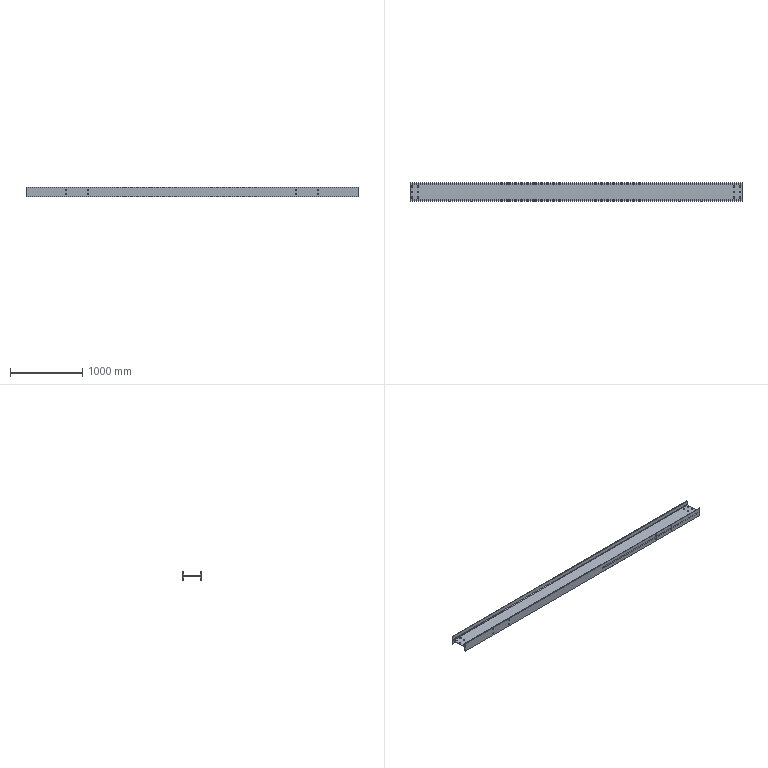Part | STEP file | Powder bin main beam 5 body_Default<As Machined> | 1 solid | 58 faces | box 4586 x 250 x 125 mm | volume 16921020 mm3 | cylinder 44 | plane 14 | commonest cylinder face diameters 19 x24 15 x16 16 x4